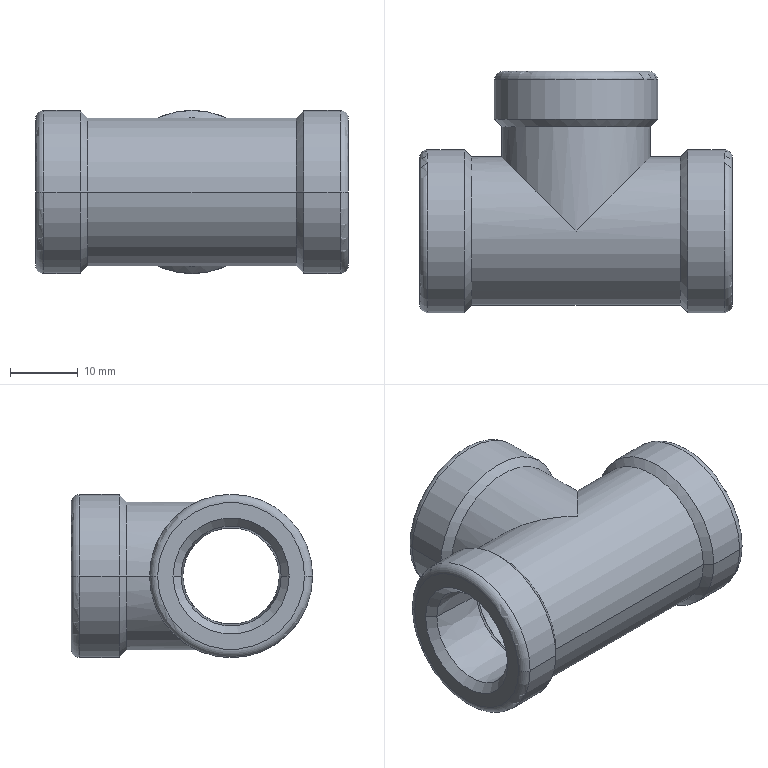Part | NX | 1 solid | 57 faces | box 46 x 35.5 x 24 mm | volume 12025 mm3 | cone 24 | cylinder 21 | torus 6 | plane 6 | commonest cylinder face diameters 24 x6 16.674 x5 16.381 x4 21.818 x4 16.456 x2